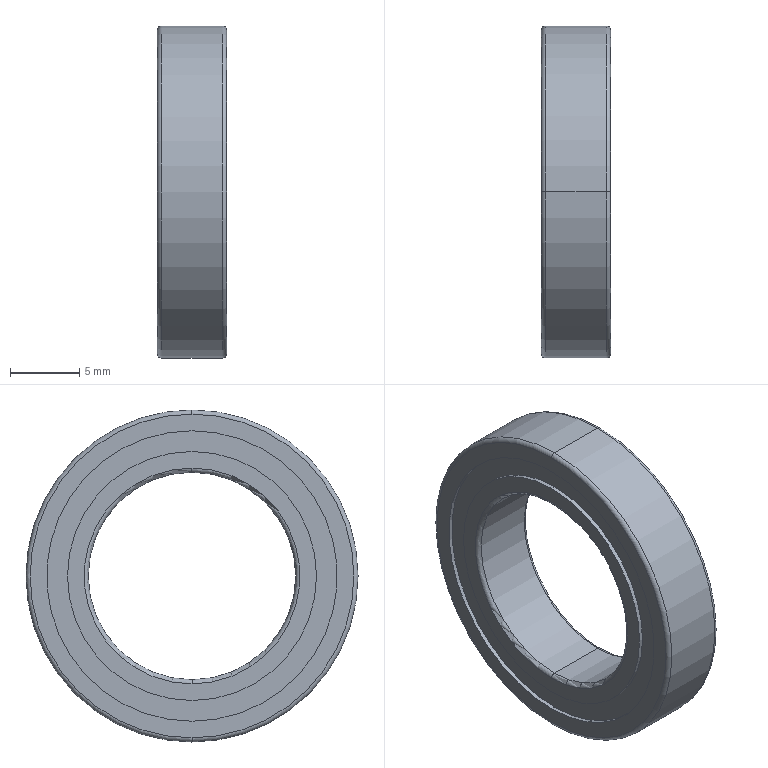Part | STEP file | 61802ZZ_Rolling bearings 61802 GB 276-94 | 1 solid | 169 faces | box 5 x 24 x 24 mm | volume 1110 mm3 | torus 89 | sphere 52 | cylinder 20 | plane 8 | commonest cylinder face diameters 18 x8 21 x8 15 x2 24 x2